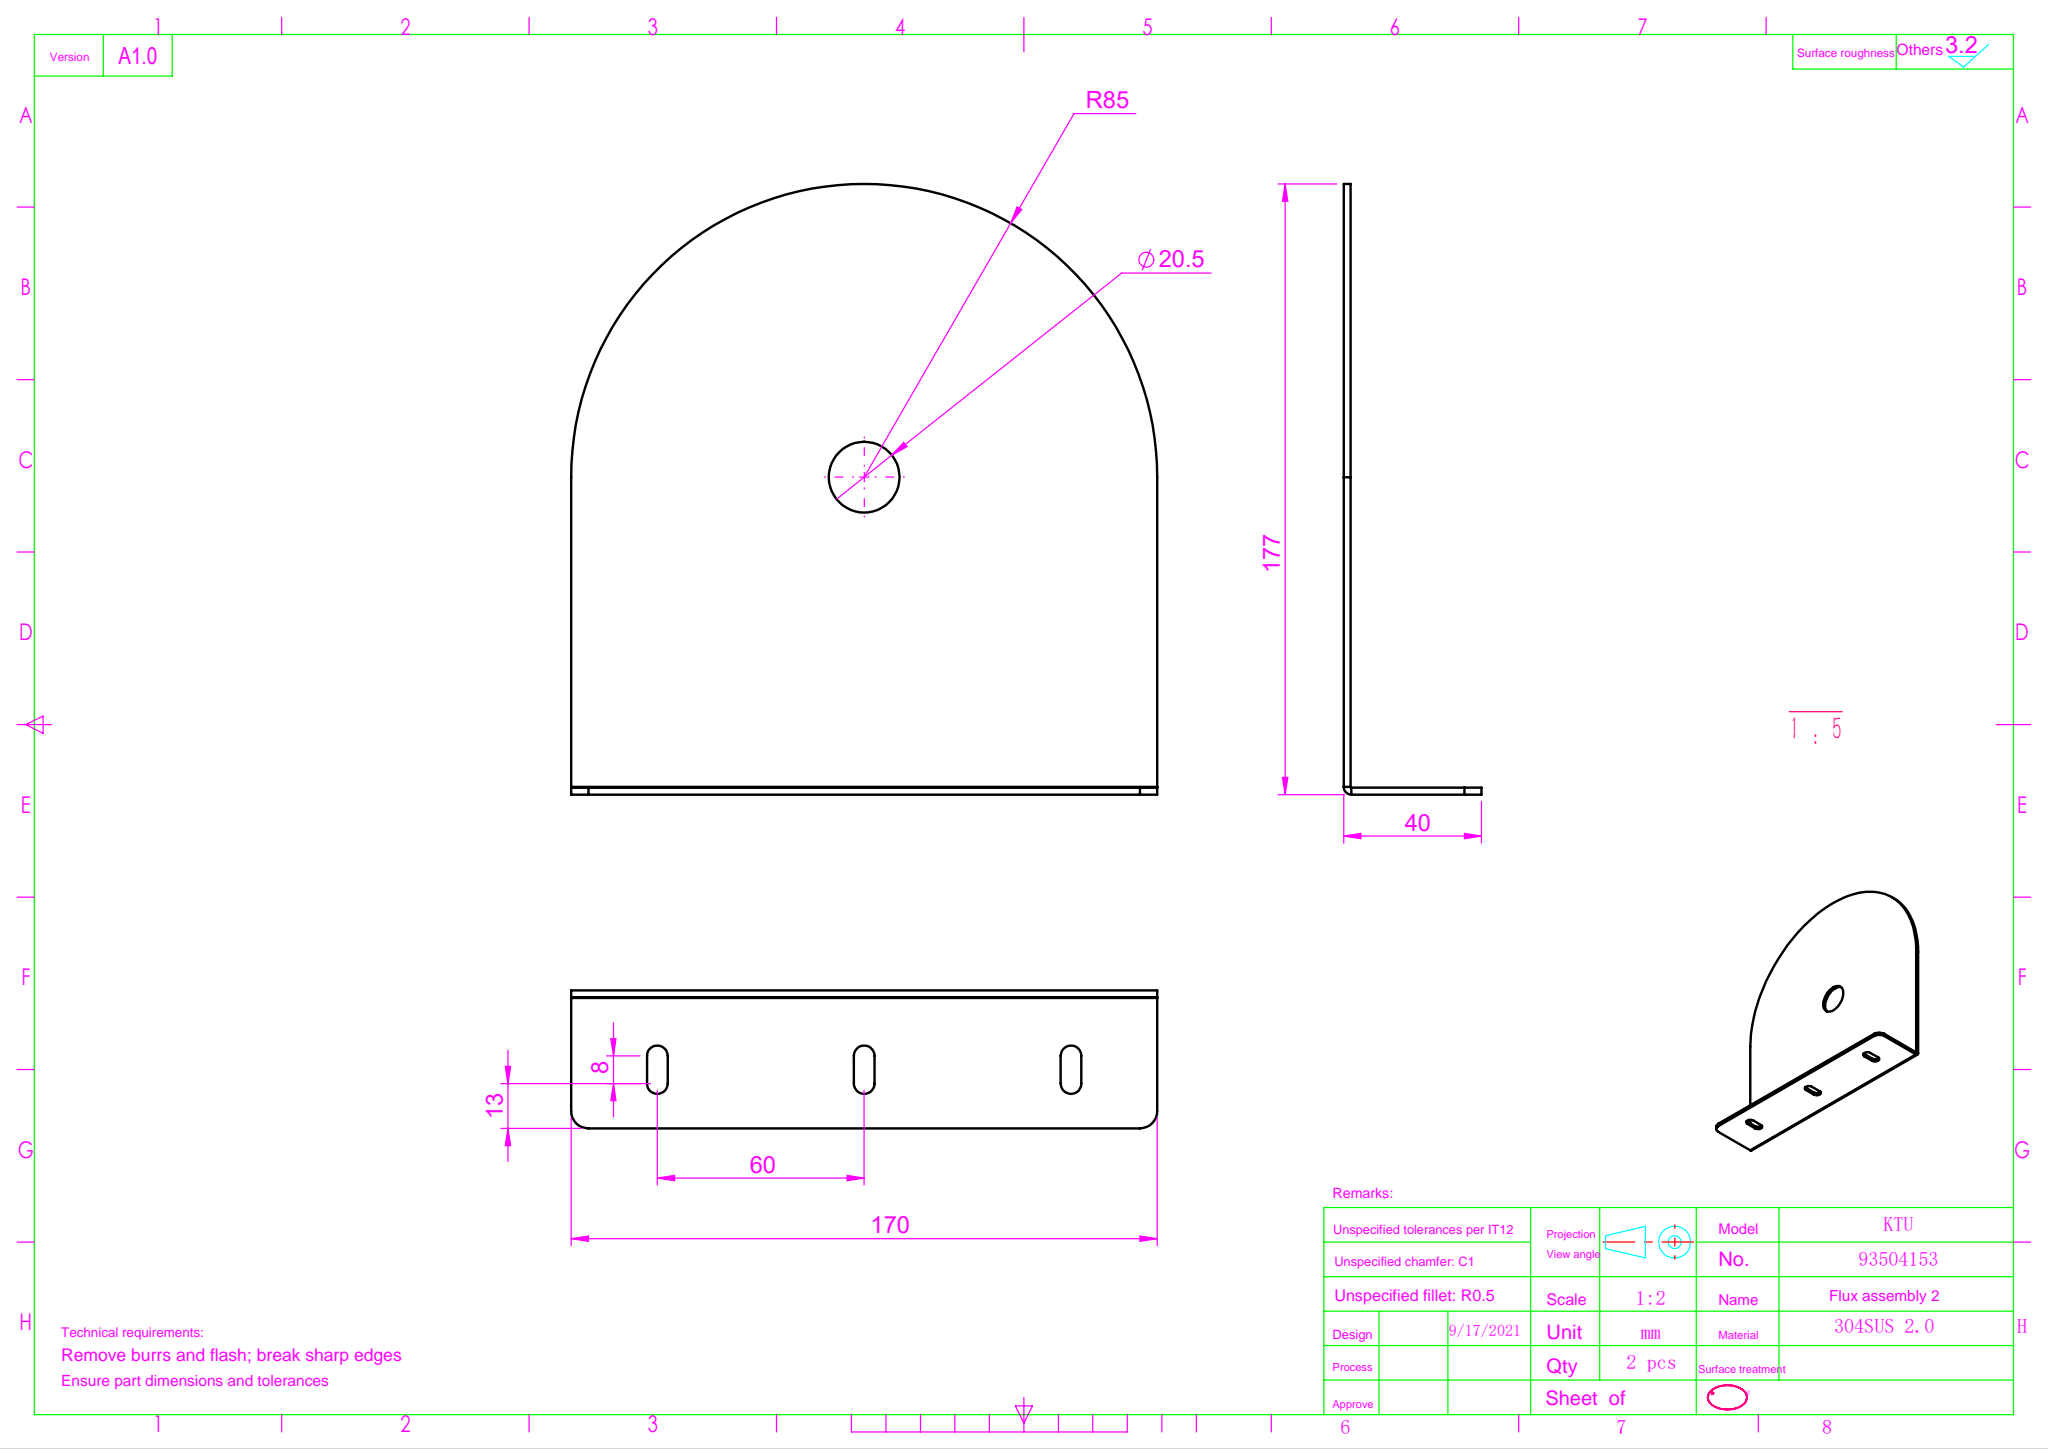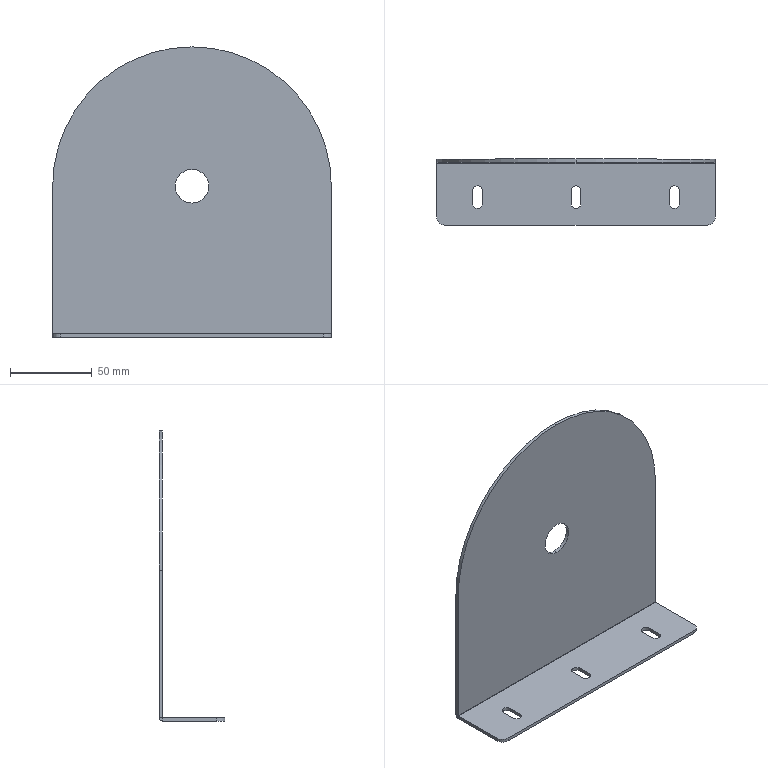Part | SolidWorks | features EdgeFlange 1, Fillet 1, FlatPattern 1, ICE 1, LPattern 1, SMBaseFlange 1, SheetMetal 1 | 1 solid | 31 faces | box 170 x 40 x 177 mm | volume 65584 mm3 | plane 17 | cylinder 14 | commonest cylinder face diameters 6 x6 10 x2 20.5 x2 170 x2 0.4 x1 4.4 x1
STEP:
#1=CARTESIAN_POINT('',(0.,-2.,-10.25));
#2=VERTEX_POINT('',#1);
#3=CARTESIAN_POINT('',(0.,-2.,10.25));
#4=VERTEX_POINT('',#3);
#5=CARTESIAN_POINT('',(0.,-2.,0.));
#6=DIRECTION('',(0.,1.,0.));
#7=DIRECTION('',(0.,0.,1.));
#8=AXIS2_PLACEMENT_3D('',#5,#6,#7);
#9=CIRCLE('',#8,10.25);
#10=EDGE_CURVE('',#2,#4,#9,.T.);
#11=ORIENTED_EDGE('',*,*,#10,.F.);
#12=CARTESIAN_POINT('',(0.,0.,-10.25));
#13=VERTEX_POINT('',#12);
#14=CARTESIAN_POINT('',(0.,-2.,-10.25));
#15=DIRECTION('',(0.,1.,0.));
#16=VECTOR('',#15,1000.);
#17=LINE('',#14,#16);
#18=EDGE_CURVE('',#2,#13,#17,.T.);
#19=ORIENTED_EDGE('',*,*,#18,.T.);
#20=CARTESIAN_POINT('',(0.,0.,10.25));
#21=VERTEX_POINT('',#20);
#22=CARTESIAN_POINT('',(0.,0.,0.));
#23=DIRECTION('',(0.,1.,0.));
#24=DIRECTION('',(0.,0.,1.));
#25=AXIS2_PLACEMENT_3D('',#22,#23,#24);
#26=CIRCLE('',#25,10.25);
#27=EDGE_CURVE('',#13,#21,#26,.T.);
#28=ORIENTED_EDGE('',*,*,#27,.T.);
#29=CARTESIAN_POINT('',(0.,-2.,10.25));
#30=DIRECTION('',(0.,1.,0.));
#31=VECTOR('',#30,1000.);
#32=LINE('',#29,#31);
#33=EDGE_CURVE('',#4,#21,#32,.T.);
#34=ORIENTED_EDGE('',*,*,#33,.F.);
#35=EDGE_LOOP('',(#11,#19,#28,#34));
#36=FACE_OUTER_BOUND('',#35,.T.);
#37=CARTESIAN_POINT('',(0.,-2.,0.));
#38=DIRECTION('',(0.,1.,0.));
#39=DIRECTION('',(0.,0.,1.));
#40=AXIS2_PLACEMENT_3D('',#37,#38,#39);
#41=CYLINDRICAL_SURFACE('',#40,10.25);
#42=ADVANCED_FACE('',(#36),#41,.F.);
#43=CARTESIAN_POINT('',(-85.,-2.,0.));
#44=VERTEX_POINT('',#43);
#45=CARTESIAN_POINT('',(0.,-2.,85.));
#46=VERTEX_POINT('',#45);
#47=CARTESIAN_POINT('',(0.,-2.,0.));
#48=DIRECTION('',(0.,1.,0.));
#49=DIRECTION('',(0.,0.,1.));
#50=AXIS2_PLACEMENT_3D('',#47,#48,#49);
#51=CIRCLE('',#50,85.);
#52=EDGE_CURVE('',#44,#46,#51,.T.);
#53=ORIENTED_EDGE('',*,*,#52,.T.);
#54=CARTESIAN_POINT('',(0.,0.,85.));
#55=VERTEX_POINT('',#54);
#56=CARTESIAN_POINT('',(0.,-2.,85.));
#57=DIRECTION('',(0.,1.,0.));
#58=VECTOR('',#57,1000.);
#59=LINE('',#56,#58);
#60=EDGE_CURVE('',#46,#55,#59,.T.);
#61=ORIENTED_EDGE('',*,*,#60,.T.);
#62=CARTESIAN_POINT('',(-85.,0.,0.));
#63=VERTEX_POINT('',#62);
#64=CARTESIAN_POINT('',(0.,0.,0.));
#65=DIRECTION('',(0.,1.,0.));
#66=DIRECTION('',(0.,0.,1.));
#67=AXIS2_PLACEMENT_3D('',#64,#65,#66);
#68=CIRCLE('',#67,85.);
#69=EDGE_CURVE('',#63,#55,#68,.T.);
#70=ORIENTED_EDGE('',*,*,#69,.F.);
#71=CARTESIAN_POINT('',(-85.,-2.,0.));
#72=DIRECTION('',(0.,1.,0.));
#73=VECTOR('',#72,1000.);
#74=LINE('',#71,#73);
#75=EDGE_CURVE('',#44,#63,#74,.T.);
#76=ORIENTED_EDGE('',*,*,#75,.F.);
#77=EDGE_LOOP('',(#53,#61,#70,#76));
#78=FACE_OUTER_BOUND('',#77,.T.);
#79=CARTESIAN_POINT('',(0.,-2.,0.));
#80=DIRECTION('',(0.,1.,0.));
#81=DIRECTION('',(0.,0.,1.));
#82=AXIS2_PLACEMENT_3D('',#79,#80,#81);
#83=CYLINDRICAL_SURFACE('',#82,85.);
#84=ADVANCED_FACE('',(#78),#83,.T.);
#85=CARTESIAN_POINT('',(85.,-2.,0.));
#86=VERTEX_POINT('',#85);
#87=CARTESIAN_POINT('',(85.,-2.,-89.8));
#88=VERTEX_POINT('',#87);
#89=CARTESIAN_POINT('',(85.,-2.,-92.));
#90=DIRECTION('',(0.,0.,-1.));
#91=VECTOR('',#90,1000.);
#92=LINE('',#89,#91);
#93=EDGE_CURVE('',#86,#88,#92,.T.);
#94=ORIENTED_EDGE('',*,*,#93,.T.);
#95=CARTESIAN_POINT('',(85.,0.,-89.8));
#96=VERTEX_POINT('',#95);
#97=CARTESIAN_POINT('',(85.,-2.,-89.8));
#98=DIRECTION('',(0.,1.,0.));
#99=VECTOR('',#98,1000.);
#100=LINE('',#97,#99);
#101=EDGE_CURVE('',#88,#96,#100,.T.);
#102=ORIENTED_EDGE('',*,*,#101,.T.);
#103=CARTESIAN_POINT('',(85.,0.,0.));
#104=VERTEX_POINT('',#103);
#105=CARTESIAN_POINT('',(85.,0.,-92.));
#106=DIRECTION('',(0.,0.,-1.));
#107=VECTOR('',#106,1000.);
#108=LINE('',#105,#107);
#109=EDGE_CURVE('',#104,#96,#108,.T.);
#110=ORIENTED_EDGE('',*,*,#109,.F.);
#111=CARTESIAN_POINT('',(85.,-2.,0.));
#112=DIRECTION('',(0.,1.,0.));
#113=VECTOR('',#112,1000.);
#114=LINE('',#111,#113);
#115=EDGE_CURVE('',#86,#104,#114,.T.);
#116=ORIENTED_EDGE('',*,*,#115,.F.);
#117=EDGE_LOOP('',(#94,#102,#110,#116));
#118=FACE_OUTER_BOUND('',#117,.T.);
#119=CARTESIAN_POINT('',(85.,-2.,-92.));
#120=DIRECTION('',(1.,0.,0.));
#121=DIRECTION('',(0.,0.,-1.));
#122=AXIS2_PLACEMENT_3D('',#119,#120,#121);
#123=PLANE('',#122);
#124=ADVANCED_FACE('',(#118),#123,.T.);
#125=CARTESIAN_POINT('',(0.,-2.,0.));
#126=DIRECTION('',(0.,1.,0.));
#127=DIRECTION('',(0.,0.,1.));
#128=AXIS2_PLACEMENT_3D('',#125,#126,#127);
#129=CIRCLE('',#128,10.25);
#130=EDGE_CURVE('',#4,#2,#129,.T.);
#131=ORIENTED_EDGE('',*,*,#130,.T.);
#132=ORIENTED_EDGE('',*,*,#10,.T.);
#133=EDGE_LOOP('',(#131,#132));
#134=FACE_BOUND('',#133,.T.);
#135=CARTESIAN_POINT('',(-85.,-2.,-89.8));
#136=VERTEX_POINT('',#135);
#137=CARTESIAN_POINT('',(85.,-2.,-89.8));
#138=DIRECTION('',(-1.,0.,0.));
#139=VECTOR('',#138,1000.);
#140=LINE('',#137,#139);
#141=EDGE_CURVE('',#88,#136,#140,.T.);
#142=ORIENTED_EDGE('',*,*,#141,.F.);
#143=ORIENTED_EDGE('',*,*,#93,.F.);
#144=CARTESIAN_POINT('',(0.,-2.,0.));
#145=DIRECTION('',(0.,1.,0.));
#146=DIRECTION('',(0.,0.,1.));
#147=AXIS2_PLACEMENT_3D('',#144,#145,#146);
#148=CIRCLE('',#147,85.);
#149=EDGE_CURVE('',#46,#86,#148,.T.);
#150=ORIENTED_EDGE('',*,*,#149,.F.);
#151=ORIENTED_EDGE('',*,*,#52,.F.);
#152=CARTESIAN_POINT('',(-85.,-2.,0.));
#153=DIRECTION('',(0.,0.,1.));
#154=VECTOR('',#153,1000.);
#155=LINE('',#152,#154);
#156=EDGE_CURVE('',#136,#44,#155,.T.);
#157=ORIENTED_EDGE('',*,*,#156,.F.);
#158=EDGE_LOOP('',(#142,#143,#150,#151,#157));
#159=FACE_OUTER_BOUND('',#158,.T.);
#160=CARTESIAN_POINT('',(0.,-2.,0.));
#161=DIRECTION('',(0.,1.,0.));
#162=DIRECTION('',(0.,0.,1.));
#163=AXIS2_PLACEMENT_3D('',#160,#161,#162);
#164=PLANE('',#163);
#165=ADVANCED_FACE('',(#134,#159),#164,.F.);
#166=CARTESIAN_POINT('',(0.,0.,0.));
#167=DIRECTION('',(0.,1.,0.));
#168=DIRECTION('',(0.,0.,1.));
#169=AXIS2_PLACEMENT_3D('',#166,#167,#168);
#170=CIRCLE('',#169,10.25);
#171=EDGE_CURVE('',#21,#13,#170,.T.);
#172=ORIENTED_EDGE('',*,*,#171,.F.);
#173=ORIENTED_EDGE('',*,*,#27,.F.);
#174=EDGE_LOOP('',(#172,#173));
#175=FACE_BOUND('',#174,.T.);
#176=ORIENTED_EDGE('',*,*,#109,.T.);
#177=CARTESIAN_POINT('',(-85.,0.,-89.8));
#178=VERTEX_POINT('',#177);
#179=CARTESIAN_POINT('',(85.,0.,-89.8));
#180=DIRECTION('',(-1.,0.,0.));
#181=VECTOR('',#180,1000.);
#182=LINE('',#179,#181);
#183=EDGE_CURVE('',#96,#178,#182,.T.);
#184=ORIENTED_EDGE('',*,*,#183,.T.);
#185=CARTESIAN_POINT('',(-85.,0.,0.));
#186=DIRECTION('',(0.,0.,1.));
#187=VECTOR('',#186,1000.);
#188=LINE('',#185,#187);
#189=EDGE_CURVE('',#178,#63,#188,.T.);
#190=ORIENTED_EDGE('',*,*,#189,.T.);
#191=ORIENTED_EDGE('',*,*,#69,.T.);
#192=CARTESIAN_POINT('',(0.,0.,0.));
#193=DIRECTION('',(0.,1.,0.));
#194=DIRECTION('',(0.,0.,1.));
#195=AXIS2_PLACEMENT_3D('',#192,#193,#194);
#196=CIRCLE('',#195,85.);
#197=EDGE_CURVE('',#55,#104,#196,.T.);
#198=ORIENTED_EDGE('',*,*,#197,.T.);
#199=EDGE_LOOP('',(#176,#184,#190,#191,#198));
#200=FACE_OUTER_BOUND('',#199,.T.);
#201=CARTESIAN_POINT('',(0.,0.,0.));
#202=DIRECTION('',(0.,1.,0.));
#203=DIRECTION('',(0.,0.,1.));
#204=AXIS2_PLACEMENT_3D('',#201,#202,#203);
#205=PLANE('',#204);
#206=ADVANCED_FACE('',(#175,#200),#205,.T.);
#207=ORIENTED_EDGE('',*,*,#60,.F.);
#208=ORIENTED_EDGE('',*,*,#149,.T.);
#209=ORIENTED_EDGE('',*,*,#115,.T.);
#210=ORIENTED_EDGE('',*,*,#197,.F.);
#211=EDGE_LOOP('',(#207,#208,#209,#210));
#212=FACE_OUTER_BOUND('',#211,.T.);
#213=CARTESIAN_POINT('',(0.,-2.,0.));
#214=DIRECTION('',(0.,1.,0.));
#215=DIRECTION('',(0.,0.,1.));
#216=AXIS2_PLACEMENT_3D('',#213,#214,#215);
#217=CYLINDRICAL_SURFACE('',#216,85.);
#218=ADVANCED_FACE('',(#212),#217,.T.);
#219=CARTESIAN_POINT('',(-85.,-2.,-89.8));
#220=DIRECTION('',(0.,1.,0.));
#221=VECTOR('',#220,1000.);
#222=LINE('',#219,#221);
#223=EDGE_CURVE('',#136,#178,#222,.T.);
#224=ORIENTED_EDGE('',*,*,#223,.F.);
#225=ORIENTED_EDGE('',*,*,#156,.T.);
#226=ORIENTED_EDGE('',*,*,#75,.T.);
#227=ORIENTED_EDGE('',*,*,#189,.F.);
#228=EDGE_LOOP('',(#224,#225,#226,#227));
#229=FACE_OUTER_BOUND('',#228,.T.);
#230=CARTESIAN_POINT('',(-85.,-2.,0.));
#231=DIRECTION('',(-1.,0.,0.));
#232=DIRECTION('',(0.,0.,1.));
#233=AXIS2_PLACEMENT_3D('',#230,#231,#232);
#234=PLANE('',#233);
#235=ADVANCED_FACE('',(#229),#234,.T.);
#236=ORIENTED_EDGE('',*,*,#18,.F.);
#237=ORIENTED_EDGE('',*,*,#130,.F.);
#238=ORIENTED_EDGE('',*,*,#33,.T.);
#239=ORIENTED_EDGE('',*,*,#171,.T.);
#240=EDGE_LOOP('',(#236,#237,#238,#239));
#241=FACE_OUTER_BOUND('',#240,.T.);
#242=CARTESIAN_POINT('',(0.,-2.,0.));
#243=DIRECTION('',(0.,1.,0.));
#244=DIRECTION('',(0.,0.,1.));
#245=AXIS2_PLACEMENT_3D('',#242,#243,#244);
#246=CYLINDRICAL_SURFACE('',#245,10.25);
#247=ADVANCED_FACE('',(#241),#246,.F.);
#248=CARTESIAN_POINT('',(-85.,-2.2,-90.));
#249=VERTEX_POINT('',#248);
#250=CARTESIAN_POINT('',(-85.,-2.2,-92.));
#251=VERTEX_POINT('',#250);
#252=CARTESIAN_POINT('',(-85.,-2.2,-92.));
#253=DIRECTION('',(0.,0.,-1.));
#254=VECTOR('',#253,1000.);
#255=LINE('',#252,#254);
#256=EDGE_CURVE('',#249,#251,#255,.T.);
#257=ORIENTED_EDGE('',*,*,#256,.F.);
#258=CARTESIAN_POINT('',(-85.,-2.2,-89.8));
#259=DIRECTION('',(-1.,0.,0.));
#260=DIRECTION('',(0.,0.,-1.));
#261=AXIS2_PLACEMENT_3D('',#258,#259,#260);
#262=CIRCLE('',#261,0.2);
#263=EDGE_CURVE('',#136,#249,#262,.T.);
#264=ORIENTED_EDGE('',*,*,#263,.F.);
#265=ORIENTED_EDGE('',*,*,#223,.T.);
#266=CARTESIAN_POINT('',(-85.,-2.2,-89.8));
#267=DIRECTION('',(-1.,0.,0.));
#268=DIRECTION('',(0.,0.,-1.));
#269=AXIS2_PLACEMENT_3D('',#266,#267,#268);
#270=CIRCLE('',#269,2.2);
#271=EDGE_CURVE('',#178,#251,#270,.T.);
#272=ORIENTED_EDGE('',*,*,#271,.T.);
#273=EDGE_LOOP('',(#257,#264,#265,#272));
#274=FACE_OUTER_BOUND('',#273,.T.);
#275=CARTESIAN_POINT('',(-85.,-2.2,-89.8));
#276=DIRECTION('',(-1.,0.,0.));
#277=DIRECTION('',(0.,0.,1.));
#278=AXIS2_PLACEMENT_3D('',#275,#276,#277);
#279=PLANE('',#278);
#280=ADVANCED_FACE('',(#274),#279,.T.);
#281=CARTESIAN_POINT('',(85.,-2.2,-90.));
#282=VERTEX_POINT('',#281);
#283=CARTESIAN_POINT('',(85.,-2.2,-89.8));
#284=DIRECTION('',(1.,0.,0.));
#285=DIRECTION('',(0.,0.,-1.));
#286=AXIS2_PLACEMENT_3D('',#283,#284,#285);
#287=CIRCLE('',#286,0.2);
#288=EDGE_CURVE('',#282,#88,#287,.T.);
#289=ORIENTED_EDGE('',*,*,#288,.F.);
#290=CARTESIAN_POINT('',(85.,-2.2,-92.));
#291=VERTEX_POINT('',#290);
#292=CARTESIAN_POINT('',(85.,-2.2,-90.));
#293=DIRECTION('',(0.,0.,-1.));
#294=VECTOR('',#293,1000.);
#295=LINE('',#292,#294);
#296=EDGE_CURVE('',#282,#291,#295,.T.);
#297=ORIENTED_EDGE('',*,*,#296,.T.);
#298=CARTESIAN_POINT('',(85.,-2.2,-89.8));
#299=DIRECTION('',(1.,0.,0.));
#300=DIRECTION('',(0.,0.,-1.));
#301=AXIS2_PLACEMENT_3D('',#298,#299,#300);
#302=CIRCLE('',#301,2.2);
#303=EDGE_CURVE('',#291,#96,#302,.T.);
#304=ORIENTED_EDGE('',*,*,#303,.T.);
#305=ORIENTED_EDGE('',*,*,#101,.F.);
#306=EDGE_LOOP('',(#289,#297,#304,#305));
#307=FACE_OUTER_BOUND('',#306,.T.);
#308=CARTESIAN_POINT('',(85.,-2.2,-89.8));
#309=DIRECTION('',(-1.,0.,0.));
#310=DIRECTION('',(0.,0.,1.));
#311=AXIS2_PLACEMENT_3D('',#308,#309,#310);
#312=PLANE('',#311);
#313=ADVANCED_FACE('',(#307),#312,.F.);
#314=ORIENTED_EDGE('',*,*,#183,.F.);
#315=ORIENTED_EDGE('',*,*,#303,.F.);
#316=CARTESIAN_POINT('',(0.,-2.2,-92.));
#317=DIRECTION('',(1.,0.,0.));
#318=VECTOR('',#317,1000.);
#319=LINE('',#316,#318);
#320=EDGE_CURVE('',#251,#291,#319,.T.);
#321=ORIENTED_EDGE('',*,*,#320,.F.);
#322=ORIENTED_EDGE('',*,*,#271,.F.);
#323=EDGE_LOOP('',(#314,#315,#321,#322));
#324=FACE_OUTER_BOUND('',#323,.T.);
#325=CARTESIAN_POINT('',(85.,-2.2,-89.8));
#326=DIRECTION('',(1.,0.,0.));
#327=DIRECTION('',(0.,0.,-1.));
#328=AXIS2_PLACEMENT_3D('',#325,#326,#327);
#329=CYLINDRICAL_SURFACE('',#328,2.2);
#330=ADVANCED_FACE('',(#324),#329,.T.);
#331=ORIENTED_EDGE('',*,*,#141,.T.);
#332=ORIENTED_EDGE('',*,*,#263,.T.);
#333=CARTESIAN_POINT('',(-85.,-2.2,-90.));
#334=DIRECTION('',(1.,0.,0.));
#335=VECTOR('',#334,1000.);
#336=LINE('',#333,#335);
#337=EDGE_CURVE('',#249,#282,#336,.T.);
#338=ORIENTED_EDGE('',*,*,#337,.T.);
#339=ORIENTED_EDGE('',*,*,#288,.T.);
#340=EDGE_LOOP('',(#331,#332,#338,#339));
#341=FACE_OUTER_BOUND('',#340,.T.);
#342=CARTESIAN_POINT('',(85.,-2.2,-89.8));
#343=DIRECTION('',(1.,0.,0.));
#344=DIRECTION('',(0.,0.,-1.));
#345=AXIS2_PLACEMENT_3D('',#342,#343,#344);
#346=CYLINDRICAL_SURFACE('',#345,0.2);
#347=ADVANCED_FACE('',(#341),#346,.F.);
#348=CARTESIAN_POINT('',(85.,-35.,-90.));
#349=VERTEX_POINT('',#348);
#350=CARTESIAN_POINT('',(85.,0.,-90.));
#351=DIRECTION('',(0.,1.,0.));
#352=VECTOR('',#351,1000.);
#353=LINE('',#350,#352);
#354=EDGE_CURVE('',#349,#282,#353,.T.);
#355=ORIENTED_EDGE('',*,*,#354,.F.);
#356=CARTESIAN_POINT('',(85.,-35.,-92.));
#357=VERTEX_POINT('',#356);
#358=CARTESIAN_POINT('',(85.,-35.,-92.));
#359=DIRECTION('',(0.,0.,-1.));
#360=VECTOR('',#359,1000.);
#361=LINE('',#358,#360);
#362=EDGE_CURVE('',#349,#357,#361,.T.);
#363=ORIENTED_EDGE('',*,*,#362,.T.);
#364=CARTESIAN_POINT('',(85.,-2.,-92.));
#365=DIRECTION('',(0.,1.,0.));
#366=VECTOR('',#365,1000.);
#367=LINE('',#364,#366);
#368=EDGE_CURVE('',#357,#291,#367,.T.);
#369=ORIENTED_EDGE('',*,*,#368,.T.);
#370=ORIENTED_EDGE('',*,*,#296,.F.);
#371=EDGE_LOOP('',(#355,#363,#369,#370));
#372=FACE_OUTER_BOUND('',#371,.T.);
#373=CARTESIAN_POINT('',(85.,-2.,-92.));
#374=DIRECTION('',(1.,0.,0.));
#375=DIRECTION('',(0.,0.,-1.));
#376=AXIS2_PLACEMENT_3D('',#373,#374,#375);
#377=PLANE('',#376);
#378=ADVANCED_FACE('',(#372),#377,.T.);
#379=CARTESIAN_POINT('',(-85.,-35.,-92.));
#380=VERTEX_POINT('',#379);
#381=CARTESIAN_POINT('',(-85.,-40.,-92.));
#382=DIRECTION('',(0.,-1.,0.));
#383=VECTOR('',#382,1000.);
#384=LINE('',#381,#383);
#385=EDGE_CURVE('',#251,#380,#384,.T.);
#386=ORIENTED_EDGE('',*,*,#385,.T.);
#387=CARTESIAN_POINT('',(-85.,-35.,-90.));
#388=VERTEX_POINT('',#387);
#389=CARTESIAN_POINT('',(-85.,-35.,-92.));
#390=DIRECTION('',(0.,0.,1.));
#391=VECTOR('',#390,1000.);
#392=LINE('',#389,#391);
#393=EDGE_CURVE('',#380,#388,#392,.T.);
#394=ORIENTED_EDGE('',*,*,#393,.T.);
#395=CARTESIAN_POINT('',(-85.,0.,-90.));
#396=DIRECTION('',(0.,-1.,0.));
#397=VECTOR('',#396,1000.);
#398=LINE('',#395,#397);
#399=EDGE_CURVE('',#249,#388,#398,.T.);
#400=ORIENTED_EDGE('',*,*,#399,.F.);
#401=ORIENTED_EDGE('',*,*,#256,.T.);
#402=EDGE_LOOP('',(#386,#394,#400,#401));
#403=FACE_OUTER_BOUND('',#402,.T.);
#404=CARTESIAN_POINT('',(-85.,-40.,-92.));
#405=DIRECTION('',(-1.,0.,0.));
#406=DIRECTION('',(0.,0.,1.));
#407=AXIS2_PLACEMENT_3D('',#404,#405,#406);
#408=PLANE('',#407);
#409=ADVANCED_FACE('',(#403),#408,.T.);
#410=CARTESIAN_POINT('',(-57.,-19.,-92.));
#411=VERTEX_POINT('',#410);
#412=CARTESIAN_POINT('',(-63.,-19.,-92.));
#413=VERTEX_POINT('',#412);
#414=CARTESIAN_POINT('',(-60.,-19.,-92.));
#415=DIRECTION('',(0.,0.,1.));
#416=DIRECTION('',(1.,0.,0.));
#417=AXIS2_PLACEMENT_3D('',#414,#415,#416);
#418=CIRCLE('',#417,3.);
#419=EDGE_CURVE('',#411,#413,#418,.T.);
#420=ORIENTED_EDGE('',*,*,#419,.T.);
#421=CARTESIAN_POINT('',(-63.,-27.,-92.));
#422=VERTEX_POINT('',#421);
#423=CARTESIAN_POINT('',(-63.,-19.,-92.));
#424=DIRECTION('',(0.,-1.,0.));
#425=VECTOR('',#424,1000.);
#426=LINE('',#423,#425);
#427=EDGE_CURVE('',#413,#422,#426,.T.);
#428=ORIENTED_EDGE('',*,*,#427,.T.);
#429=CARTESIAN_POINT('',(-57.,-27.,-92.));
#430=VERTEX_POINT('',#429);
#431=CARTESIAN_POINT('',(-60.,-27.,-92.));
#432=DIRECTION('',(0.,0.,1.));
#433=DIRECTION('',(1.,0.,0.));
#434=AXIS2_PLACEMENT_3D('',#431,#432,#433);
#435=CIRCLE('',#434,3.);
#436=EDGE_CURVE('',#422,#430,#435,.T.);
#437=ORIENTED_EDGE('',*,*,#436,.T.);
#438=CARTESIAN_POINT('',(-57.,-19.,-92.));
#439=DIRECTION('',(0.,1.,0.));
#440=VECTOR('',#439,1000.);
#441=LINE('',#438,#440);
#442=EDGE_CURVE('',#430,#411,#441,.T.);
#443=ORIENTED_EDGE('',*,*,#442,.T.);
#444=EDGE_LOOP('',(#420,#428,#437,#443));
#445=FACE_BOUND('',#444,.T.);
#446=CARTESIAN_POINT('',(63.,-19.,-92.));
#447=VERTEX_POINT('',#446);
#448=CARTESIAN_POINT('',(57.,-19.,-92.));
#449=VERTEX_POINT('',#448);
#450=CARTESIAN_POINT('',(60.,-19.,-92.));
#451=DIRECTION('',(0.,0.,1.));
#452=DIRECTION('',(1.,0.,0.));
#453=AXIS2_PLACEMENT_3D('',#450,#451,#452);
#454=CIRCLE('',#453,3.);
#455=EDGE_CURVE('',#447,#449,#454,.T.);
#456=ORIENTED_EDGE('',*,*,#455,.T.);
#457=CARTESIAN_POINT('',(57.,-27.,-92.));
#458=VERTEX_POINT('',#457);
#459=CARTESIAN_POINT('',(57.,-19.,-92.));
#460=DIRECTION('',(0.,-1.,0.));
#461=VECTOR('',#460,1000.);
#462=LINE('',#459,#461);
#463=EDGE_CURVE('',#449,#458,#462,.T.);
#464=ORIENTED_EDGE('',*,*,#463,.T.);
#465=CARTESIAN_POINT('',(63.,-27.,-92.));
#466=VERTEX_POINT('',#465);
#467=CARTESIAN_POINT('',(60.,-27.,-92.));
#468=DIRECTION('',(0.,0.,1.));
#469=DIRECTION('',(1.,0.,0.));
#470=AXIS2_PLACEMENT_3D('',#467,#468,#469);
#471=CIRCLE('',#470,3.);
#472=EDGE_CURVE('',#458,#466,#471,.T.);
#473=ORIENTED_EDGE('',*,*,#472,.T.);
#474=CARTESIAN_POINT('',(63.,-19.,-92.));
#475=DIRECTION('',(0.,1.,0.));
#476=VECTOR('',#475,1000.);
#477=LINE('',#474,#476);
#478=EDGE_CURVE('',#466,#447,#477,.T.);
#479=ORIENTED_EDGE('',*,*,#478,.T.);
#480=EDGE_LOOP('',(#456,#464,#473,#479));
#481=FACE_BOUND('',#480,.T.);
#482=CARTESIAN_POINT('',(3.,-19.,-92.));
#483=VERTEX_POINT('',#482);
#484=CARTESIAN_POINT('',(-3.,-19.,-92.));
#485=VERTEX_POINT('',#484);
#486=CARTESIAN_POINT('',(0.,-19.,-92.));
#487=DIRECTION('',(0.,0.,1.));
#488=DIRECTION('',(1.,0.,0.));
#489=AXIS2_PLACEMENT_3D('',#486,#487,#488);
#490=CIRCLE('',#489,3.);
#491=EDGE_CURVE('',#483,#485,#490,.T.);
#492=ORIENTED_EDGE('',*,*,#491,.T.);
#493=CARTESIAN_POINT('',(-3.,-27.,-92.));
#494=VERTEX_POINT('',#493);
#495=CARTESIAN_POINT('',(-3.,-19.,-92.));
#496=DIRECTION('',(0.,-1.,0.));
#497=VECTOR('',#496,1000.);
#498=LINE('',#495,#497);
#499=EDGE_CURVE('',#485,#494,#498,.T.);
#500=ORIENTED_EDGE('',*,*,#499,.T.);
#501=CARTESIAN_POINT('',(3.,-27.,-92.));
#502=VERTEX_POINT('',#501);
#503=CARTESIAN_POINT('',(0.,-27.,-92.));
#504=DIRECTION('',(0.,0.,1.));
#505=DIRECTION('',(1.,0.,0.));
#506=AXIS2_PLACEMENT_3D('',#503,#504,#505);
#507=CIRCLE('',#506,3.);
#508=EDGE_CURVE('',#494,#502,#507,.T.);
#509=ORIENTED_EDGE('',*,*,#508,.T.);
#510=CARTESIAN_POINT('',(3.,-19.,-92.));
#511=DIRECTION('',(0.,1.,0.));
#512=VECTOR('',#511,1000.);
#513=LINE('',#510,#512);
#514=EDGE_CURVE('',#502,#483,#513,.T.);
#515=ORIENTED_EDGE('',*,*,#514,.T.);
#516=EDGE_LOOP('',(#492,#500,#509,#515));
#517=FACE_BOUND('',#516,.T.);
#518=CARTESIAN_POINT('',(-80.,-40.,-92.));
#519=VERTEX_POINT('',#518);
#520=CARTESIAN_POINT('',(80.,-40.,-92.));
#521=VERTEX_POINT('',#520);
#522=CARTESIAN_POINT('',(85.,-40.,-92.));
#523=DIRECTION('',(1.,0.,0.));
#524=VECTOR('',#523,1000.);
#525=LINE('',#522,#524);
#526=EDGE_CURVE('',#519,#521,#525,.T.);
#527=ORIENTED_EDGE('',*,*,#526,.F.);
#528=CARTESIAN_POINT('',(-80.,-35.,-92.));
#529=DIRECTION('',(0.,0.,-1.));
#530=DIRECTION('',(0.,1.,0.));
#531=AXIS2_PLACEMENT_3D('',#528,#529,#530);
#532=CIRCLE('',#531,5.);
#533=EDGE_CURVE('',#519,#380,#532,.T.);
#534=ORIENTED_EDGE('',*,*,#533,.T.);
#535=ORIENTED_EDGE('',*,*,#385,.F.);
#536=ORIENTED_EDGE('',*,*,#320,.T.);
#537=ORIENTED_EDGE('',*,*,#368,.F.);
#538=CARTESIAN_POINT('',(80.,-35.,-92.));
#539=DIRECTION('',(0.,0.,-1.));
#540=DIRECTION('',(0.,1.,0.));
#541=AXIS2_PLACEMENT_3D('',#538,#539,#540);
#542=CIRCLE('',#541,5.);
#543=EDGE_CURVE('',#357,#521,#542,.T.);
#544=ORIENTED_EDGE('',*,*,#543,.T.);
#545=EDGE_LOOP('',(#527,#534,#535,#536,#537,#544));
#546=FACE_OUTER_BOUND('',#545,.T.);
#547=CARTESIAN_POINT('',(0.,0.,-92.));
#548=DIRECTION('',(0.,0.,-1.));
#549=DIRECTION('',(0.,1.,0.));
#550=AXIS2_PLACEMENT_3D('',#547,#548,#549);
#551=PLANE('',#550);
#552=ADVANCED_FACE('',(#445,#481,#517,#546),#551,.T.);
#553=CARTESIAN_POINT('',(-63.,-19.,-90.));
#554=VERTEX_POINT('',#553);
#555=CARTESIAN_POINT('',(-63.,-27.,-90.));
#556=VERTEX_POINT('',#555);
#557=CARTESIAN_POINT('',(-63.,-19.,-90.));
#558=DIRECTION('',(0.,-1.,0.));
#559=VECTOR('',#558,1000.);
#560=LINE('',#557,#559);
#561=EDGE_CURVE('',#554,#556,#560,.T.);
#562=ORIENTED_EDGE('',*,*,#561,.F.);
#563=CARTESIAN_POINT('',(-57.,-19.,-90.));
#564=VERTEX_POINT('',#563);
#565=CARTESIAN_POINT('',(-60.,-19.,-90.));
#566=DIRECTION('',(0.,0.,1.));
#567=DIRECTION('',(1.,0.,0.));
#568=AXIS2_PLACEMENT_3D('',#565,#566,#567);
#569=CIRCLE('',#568,3.);
#570=EDGE_CURVE('',#564,#554,#569,.T.);
#571=ORIENTED_EDGE('',*,*,#570,.F.);
#572=CARTESIAN_POINT('',(-57.,-27.,-90.));
#573=VERTEX_POINT('',#572);
#574=CARTESIAN_POINT('',(-57.,-19.,-90.));
#575=DIRECTION('',(0.,1.,0.));
#576=VECTOR('',#575,1000.);
#577=LINE('',#574,#576);
#578=EDGE_CURVE('',#573,#564,#577,.T.);
#579=ORIENTED_EDGE('',*,*,#578,.F.);
#580=CARTESIAN_POINT('',(-60.,-27.,-90.));
#581=DIRECTION('',(0.,0.,1.));
#582=DIRECTION('',(1.,0.,0.));
#583=AXIS2_PLACEMENT_3D('',#580,#581,#582);
#584=CIRCLE('',#583,3.);
#585=EDGE_CURVE('',#556,#573,#584,.T.);
#586=ORIENTED_EDGE('',*,*,#585,.F.);
#587=EDGE_LOOP('',(#562,#571,#579,#586));
#588=FACE_BOUND('',#587,.T.);
#589=CARTESIAN_POINT('',(57.,-19.,-90.));
#590=VERTEX_POINT('',#589);
#591=CARTESIAN_POINT('',(57.,-27.,-90.));
#592=VERTEX_POINT('',#591);
#593=CARTESIAN_POINT('',(57.,-19.,-90.));
#594=DIRECTION('',(0.,-1.,0.));
#595=VECTOR('',#594,1000.);
#596=LINE('',#593,#595);
#597=EDGE_CURVE('',#590,#592,#596,.T.);
#598=ORIENTED_EDGE('',*,*,#597,.F.);
#599=CARTESIAN_POINT('',(63.,-19.,-90.));
#600=VERTEX_POINT('',#599);
#601=CARTESIAN_POINT('',(60.,-19.,-90.));
#602=DIRECTION('',(0.,0.,1.));
#603=DIRECTION('',(1.,0.,0.));
#604=AXIS2_PLACEMENT_3D('',#601,#602,#603);
#605=CIRCLE('',#604,3.);
#606=EDGE_CURVE('',#600,#590,#605,.T.);
#607=ORIENTED_EDGE('',*,*,#606,.F.);
#608=CARTESIAN_POINT('',(63.,-27.,-90.));
#609=VERTEX_POINT('',#608);
#610=CARTESIAN_POINT('',(63.,-19.,-90.));
#611=DIRECTION('',(0.,1.,0.));
#612=VECTOR('',#611,1000.);
#613=LINE('',#610,#612);
#614=EDGE_CURVE('',#609,#600,#613,.T.);
#615=ORIENTED_EDGE('',*,*,#614,.F.);
#616=CARTESIAN_POINT('',(60.,-27.,-90.));
#617=DIRECTION('',(0.,0.,1.));
#618=DIRECTION('',(1.,0.,0.));
#619=AXIS2_PLACEMENT_3D('',#616,#617,#618);
#620=CIRCLE('',#619,3.);
#621=EDGE_CURVE('',#592,#609,#620,.T.);
#622=ORIENTED_EDGE('',*,*,#621,.F.);
#623=EDGE_LOOP('',(#598,#607,#615,#622));
#624=FACE_BOUND('',#623,.T.);
#625=CARTESIAN_POINT('',(-3.,-19.,-90.));
#626=VERTEX_POINT('',#625);
#627=CARTESIAN_POINT('',(-3.,-27.,-90.));
#628=VERTEX_POINT('',#627);
#629=CARTESIAN_POINT('',(-3.,-19.,-90.));
#630=DIRECTION('',(0.,-1.,0.));
#631=VECTOR('',#630,1000.);
#632=LINE('',#629,#631);
#633=EDGE_CURVE('',#626,#628,#632,.T.);
#634=ORIENTED_EDGE('',*,*,#633,.F.);
#635=CARTESIAN_POINT('',(3.,-19.,-90.));
#636=VERTEX_POINT('',#635);
#637=CARTESIAN_POINT('',(0.,-19.,-90.));
#638=DIRECTION('',(0.,0.,1.));
#639=DIRECTION('',(1.,0.,0.));
#640=AXIS2_PLACEMENT_3D('',#637,#638,#639);
#641=CIRCLE('',#640,3.);
#642=EDGE_CURVE('',#636,#626,#641,.T.);
#643=ORIENTED_EDGE('',*,*,#642,.F.);
#644=CARTESIAN_POINT('',(3.,-27.,-90.));
#645=VERTEX_POINT('',#644);
#646=CARTESIAN_POINT('',(3.,-19.,-90.));
#647=DIRECTION('',(0.,1.,0.));
#648=VECTOR('',#647,1000.);
#649=LINE('',#646,#648);
#650=EDGE_CURVE('',#645,#636,#649,.T.);
#651=ORIENTED_EDGE('',*,*,#650,.F.);
#652=CARTESIAN_POINT('',(0.,-27.,-90.));
#653=DIRECTION('',(0.,0.,1.));
#654=DIRECTION('',(1.,0.,0.));
#655=AXIS2_PLACEMENT_3D('',#652,#653,#654);
#656=CIRCLE('',#655,3.);
#657=EDGE_CURVE('',#628,#645,#656,.T.);
#658=ORIENTED_EDGE('',*,*,#657,.F.);
#659=EDGE_LOOP('',(#634,#643,#651,#658));
#660=FACE_BOUND('',#659,.T.);
#661=ORIENTED_EDGE('',*,*,#399,.T.);
#662=CARTESIAN_POINT('',(-80.,-40.,-90.));
#663=VERTEX_POINT('',#662);
#664=CARTESIAN_POINT('',(-80.,-35.,-90.));
#665=DIRECTION('',(0.,0.,1.));
#666=DIRECTION('',(0.,1.,0.));
#667=AXIS2_PLACEMENT_3D('',#664,#665,#666);
#668=CIRCLE('',#667,5.);
#669=EDGE_CURVE('',#388,#663,#668,.T.);
#670=ORIENTED_EDGE('',*,*,#669,.T.);
#671=CARTESIAN_POINT('',(80.,-40.,-90.));
#672=VERTEX_POINT('',#671);
#673=CARTESIAN_POINT('',(0.,-40.,-90.));
#674=DIRECTION('',(1.,0.,0.));
#675=VECTOR('',#674,1000.);
#676=LINE('',#673,#675);
#677=EDGE_CURVE('',#663,#672,#676,.T.);
#678=ORIENTED_EDGE('',*,*,#677,.T.);
#679=CARTESIAN_POINT('',(80.,-35.,-90.));
#680=DIRECTION('',(0.,0.,1.));
#681=DIRECTION('',(0.,1.,0.));
#682=AXIS2_PLACEMENT_3D('',#679,#680,#681);
#683=CIRCLE('',#682,5.);
#684=EDGE_CURVE('',#672,#349,#683,.T.);
#685=ORIENTED_EDGE('',*,*,#684,.T.);
#686=ORIENTED_EDGE('',*,*,#354,.T.);
#687=ORIENTED_EDGE('',*,*,#337,.F.);
#688=EDGE_LOOP('',(#661,#670,#678,#685,#686,#687));
#689=FACE_OUTER_BOUND('',#688,.T.);
#690=CARTESIAN_POINT('',(0.,0.,-90.));
#691=DIRECTION('',(0.,0.,-1.));
#692=DIRECTION('',(0.,1.,0.));
#693=AXIS2_PLACEMENT_3D('',#690,#691,#692);
#694=PLANE('',#693);
#695=ADVANCED_FACE('',(#588,#624,#660,#689),#694,.F.);
#696=ORIENTED_EDGE('',*,*,#677,.F.);
#697=CARTESIAN_POINT('',(-80.,-40.,-92.));
#698=DIRECTION('',(0.,0.,-1.));
#699=VECTOR('',#698,1000.);
#700=LINE('',#697,#699);
#701=EDGE_CURVE('',#663,#519,#700,.T.);
#702=ORIENTED_EDGE('',*,*,#701,.T.);
#703=ORIENTED_EDGE('',*,*,#526,.T.);
#704=CARTESIAN_POINT('',(80.,-40.,-92.));
#705=DIRECTION('',(0.,0.,1.));
#706=VECTOR('',#705,1000.);
#707=LINE('',#704,#706);
#708=EDGE_CURVE('',#521,#672,#707,.T.);
#709=ORIENTED_EDGE('',*,*,#708,.T.);
#710=EDGE_LOOP('',(#696,#702,#703,#709));
#711=FACE_OUTER_BOUND('',#710,.T.);
#712=CARTESIAN_POINT('',(85.,-40.,-92.));
#713=DIRECTION('',(0.,-1.,0.));
#714=DIRECTION('',(0.,0.,-1.));
#715=AXIS2_PLACEMENT_3D('',#712,#713,#714);
#716=PLANE('',#715);
#717=ADVANCED_FACE('',(#711),#716,.T.);
#718=ORIENTED_EDGE('',*,*,#642,.T.);
#719=CARTESIAN_POINT('',(-3.,-19.,-92.));
#720=DIRECTION('',(0.,0.,1.));
#721=VECTOR('',#720,1000.);
#722=LINE('',#719,#721);
#723=EDGE_CURVE('',#485,#626,#722,.T.);
#724=ORIENTED_EDGE('',*,*,#723,.F.);
#725=ORIENTED_EDGE('',*,*,#491,.F.);
#726=CARTESIAN_POINT('',(3.,-19.,-92.));
#727=DIRECTION('',(0.,0.,1.));
#728=VECTOR('',#727,1000.);
#729=LINE('',#726,#728);
#730=EDGE_CURVE('',#483,#636,#729,.T.);
#731=ORIENTED_EDGE('',*,*,#730,.T.);
#732=EDGE_LOOP('',(#718,#724,#725,#731));
#733=FACE_OUTER_BOUND('',#732,.T.);
#734=CARTESIAN_POINT('',(0.,-19.,-92.));
#735=DIRECTION('',(0.,0.,1.));
#736=DIRECTION('',(1.,0.,0.));
#737=AXIS2_PLACEMENT_3D('',#734,#735,#736);
#738=CYLINDRICAL_SURFACE('',#737,3.);
#739=ADVANCED_FACE('',(#733),#738,.F.);
#740=ORIENTED_EDGE('',*,*,#650,.T.);
#741=ORIENTED_EDGE('',*,*,#730,.F.);
#742=ORIENTED_EDGE('',*,*,#514,.F.);
#743=CARTESIAN_POINT('',(3.,-27.,-92.));
#744=DIRECTION('',(0.,0.,1.));
#745=VECTOR('',#744,1000.);
#746=LINE('',#743,#745);
#747=EDGE_CURVE('',#502,#645,#746,.T.);
#748=ORIENTED_EDGE('',*,*,#747,.T.);
#749=EDGE_LOOP('',(#740,#741,#742,#748));
#750=FACE_OUTER_BOUND('',#749,.T.);
#751=CARTESIAN_POINT('',(3.,-19.,-92.));
#752=DIRECTION('',(1.,0.,0.));
#753=DIRECTION('',(0.,1.,0.));
#754=AXIS2_PLACEMENT_3D('',#751,#752,#753);
#755=PLANE('',#754);
#756=ADVANCED_FACE('',(#750),#755,.F.);
#757=ORIENTED_EDGE('',*,*,#657,.T.);
#758=ORIENTED_EDGE('',*,*,#747,.F.);
#759=ORIENTED_EDGE('',*,*,#508,.F.);
#760=CARTESIAN_POINT('',(-3.,-27.,-92.));
#761=DIRECTION('',(0.,0.,1.));
#762=VECTOR('',#761,1000.);
#763=LINE('',#760,#762);
#764=EDGE_CURVE('',#494,#628,#763,.T.);
#765=ORIENTED_EDGE('',*,*,#764,.T.);
#766=EDGE_LOOP('',(#757,#758,#759,#765));
#767=FACE_OUTER_BOUND('',#766,.T.);
#768=CARTESIAN_POINT('',(0.,-27.,-92.));
#769=DIRECTION('',(0.,0.,1.));
#770=DIRECTION('',(1.,0.,0.));
#771=AXIS2_PLACEMENT_3D('',#768,#769,#770);
#772=CYLINDRICAL_SURFACE('',#771,3.);
#773=ADVANCED_FACE('',(#767),#772,.F.);
#774=ORIENTED_EDGE('',*,*,#633,.T.);
#775=ORIENTED_EDGE('',*,*,#764,.F.);
#776=ORIENTED_EDGE('',*,*,#499,.F.);
#777=ORIENTED_EDGE('',*,*,#723,.T.);
#778=EDGE_LOOP('',(#774,#775,#776,#777));
#779=FACE_OUTER_BOUND('',#778,.T.);
#780=CARTESIAN_POINT('',(-3.,-19.,-92.));
#781=DIRECTION('',(-1.,0.,0.));
#782=DIRECTION('',(0.,-1.,0.));
#783=AXIS2_PLACEMENT_3D('',#780,#781,#782);
#784=PLANE('',#783);
#785=ADVANCED_FACE('',(#779),#784,.F.);
#786=ORIENTED_EDGE('',*,*,#606,.T.);
#787=CARTESIAN_POINT('',(57.,-19.,-92.));
#788=DIRECTION('',(0.,0.,1.));
#789=VECTOR('',#788,1000.);
#790=LINE('',#787,#789);
#791=EDGE_CURVE('',#449,#590,#790,.T.);
#792=ORIENTED_EDGE('',*,*,#791,.F.);
#793=ORIENTED_EDGE('',*,*,#455,.F.);
#794=CARTESIAN_POINT('',(63.,-19.,-92.));
#795=DIRECTION('',(0.,0.,1.));
#796=VECTOR('',#795,1000.);
#797=LINE('',#794,#796);
#798=EDGE_CURVE('',#447,#600,#797,.T.);
#799=ORIENTED_EDGE('',*,*,#798,.T.);
#800=EDGE_LOOP('',(#786,#792,#793,#799));
#801=FACE_OUTER_BOUND('',#800,.T.);
#802=CARTESIAN_POINT('',(60.,-19.,-92.));
#803=DIRECTION('',(0.,0.,1.));
#804=DIRECTION('',(1.,0.,0.));
#805=AXIS2_PLACEMENT_3D('',#802,#803,#804);
#806=CYLINDRICAL_SURFACE('',#805,3.);
#807=ADVANCED_FACE('',(#801),#806,.F.);
#808=ORIENTED_EDGE('',*,*,#614,.T.);
#809=ORIENTED_EDGE('',*,*,#798,.F.);
#810=ORIENTED_EDGE('',*,*,#478,.F.);
#811=CARTESIAN_POINT('',(63.,-27.,-92.));
#812=DIRECTION('',(0.,0.,1.));
#813=VECTOR('',#812,1000.);
#814=LINE('',#811,#813);
#815=EDGE_CURVE('',#466,#609,#814,.T.);
#816=ORIENTED_EDGE('',*,*,#815,.T.);
#817=EDGE_LOOP('',(#808,#809,#810,#816));
#818=FACE_OUTER_BOUND('',#817,.T.);
#819=CARTESIAN_POINT('',(63.,-19.,-92.));
#820=DIRECTION('',(1.,0.,0.));
#821=DIRECTION('',(0.,1.,0.));
#822=AXIS2_PLACEMENT_3D('',#819,#820,#821);
#823=PLANE('',#822);
#824=ADVANCED_FACE('',(#818),#823,.F.);
#825=ORIENTED_EDGE('',*,*,#621,.T.);
#826=ORIENTED_EDGE('',*,*,#815,.F.);
#827=ORIENTED_EDGE('',*,*,#472,.F.);
#828=CARTESIAN_POINT('',(57.,-27.,-92.));
#829=DIRECTION('',(0.,0.,1.));
#830=VECTOR('',#829,1000.);
#831=LINE('',#828,#830);
#832=EDGE_CURVE('',#458,#592,#831,.T.);
#833=ORIENTED_EDGE('',*,*,#832,.T.);
#834=EDGE_LOOP('',(#825,#826,#827,#833));
#835=FACE_OUTER_BOUND('',#834,.T.);
#836=CARTESIAN_POINT('',(60.,-27.,-92.));
#837=DIRECTION('',(0.,0.,1.));
#838=DIRECTION('',(1.,0.,0.));
#839=AXIS2_PLACEMENT_3D('',#836,#837,#838);
#840=CYLINDRICAL_SURFACE('',#839,3.);
#841=ADVANCED_FACE('',(#835),#840,.F.);
#842=ORIENTED_EDGE('',*,*,#597,.T.);
#843=ORIENTED_EDGE('',*,*,#832,.F.);
#844=ORIENTED_EDGE('',*,*,#463,.F.);
#845=ORIENTED_EDGE('',*,*,#791,.T.);
#846=EDGE_LOOP('',(#842,#843,#844,#845));
#847=FACE_OUTER_BOUND('',#846,.T.);
#848=CARTESIAN_POINT('',(57.,-19.,-92.));
#849=DIRECTION('',(-1.,0.,0.));
#850=DIRECTION('',(0.,-1.,0.));
#851=AXIS2_PLACEMENT_3D('',#848,#849,#850);
#852=PLANE('',#851);
#853=ADVANCED_FACE('',(#847),#852,.F.);
#854=ORIENTED_EDGE('',*,*,#570,.T.);
#855=CARTESIAN_POINT('',(-63.,-19.,-92.));
#856=DIRECTION('',(0.,0.,1.));
#857=VECTOR('',#856,1000.);
#858=LINE('',#855,#857);
#859=EDGE_CURVE('',#413,#554,#858,.T.);
#860=ORIENTED_EDGE('',*,*,#859,.F.);
#861=ORIENTED_EDGE('',*,*,#419,.F.);
#862=CARTESIAN_POINT('',(-57.,-19.,-92.));
#863=DIRECTION('',(0.,0.,1.));
#864=VECTOR('',#863,1000.);
#865=LINE('',#862,#864);
#866=EDGE_CURVE('',#411,#564,#865,.T.);
#867=ORIENTED_EDGE('',*,*,#866,.T.);
#868=EDGE_LOOP('',(#854,#860,#861,#867));
#869=FACE_OUTER_BOUND('',#868,.T.);
#870=CARTESIAN_POINT('',(-60.,-19.,-92.));
#871=DIRECTION('',(0.,0.,1.));
#872=DIRECTION('',(1.,0.,0.));
#873=AXIS2_PLACEMENT_3D('',#870,#871,#872);
#874=CYLINDRICAL_SURFACE('',#873,3.);
#875=ADVANCED_FACE('',(#869),#874,.F.);
#876=ORIENTED_EDGE('',*,*,#578,.T.);
#877=ORIENTED_EDGE('',*,*,#866,.F.);
#878=ORIENTED_EDGE('',*,*,#442,.F.);
#879=CARTESIAN_POINT('',(-57.,-27.,-92.));
#880=DIRECTION('',(0.,0.,1.));
#881=VECTOR('',#880,1000.);
#882=LINE('',#879,#881);
#883=EDGE_CURVE('',#430,#573,#882,.T.);
#884=ORIENTED_EDGE('',*,*,#883,.T.);
#885=EDGE_LOOP('',(#876,#877,#878,#884));
#886=FACE_OUTER_BOUND('',#885,.T.);
#887=CARTESIAN_POINT('',(-57.,-19.,-92.));
#888=DIRECTION('',(1.,0.,0.));
#889=DIRECTION('',(0.,1.,0.));
#890=AXIS2_PLACEMENT_3D('',#887,#888,#889);
#891=PLANE('',#890);
#892=ADVANCED_FACE('',(#886),#891,.F.);
#893=ORIENTED_EDGE('',*,*,#585,.T.);
#894=ORIENTED_EDGE('',*,*,#883,.F.);
#895=ORIENTED_EDGE('',*,*,#436,.F.);
#896=CARTESIAN_POINT('',(-63.,-27.,-92.));
#897=DIRECTION('',(0.,0.,1.));
#898=VECTOR('',#897,1000.);
#899=LINE('',#896,#898);
#900=EDGE_CURVE('',#422,#556,#899,.T.);
#901=ORIENTED_EDGE('',*,*,#900,.T.);
#902=EDGE_LOOP('',(#893,#894,#895,#901));
#903=FACE_OUTER_BOUND('',#902,.T.);
#904=CARTESIAN_POINT('',(-60.,-27.,-92.));
#905=DIRECTION('',(0.,0.,1.));
#906=DIRECTION('',(1.,0.,0.));
#907=AXIS2_PLACEMENT_3D('',#904,#905,#906);
#908=CYLINDRICAL_SURFACE('',#907,3.);
#909=ADVANCED_FACE('',(#903),#908,.F.);
#910=ORIENTED_EDGE('',*,*,#561,.T.);
#911=ORIENTED_EDGE('',*,*,#900,.F.);
#912=ORIENTED_EDGE('',*,*,#427,.F.);
#913=ORIENTED_EDGE('',*,*,#859,.T.);
#914=EDGE_LOOP('',(#910,#911,#912,#913));
#915=FACE_OUTER_BOUND('',#914,.T.);
#916=CARTESIAN_POINT('',(-63.,-19.,-92.));
#917=DIRECTION('',(-1.,0.,0.));
#918=DIRECTION('',(0.,-1.,0.));
#919=AXIS2_PLACEMENT_3D('',#916,#917,#918);
#920=PLANE('',#919);
#921=ADVANCED_FACE('',(#915),#920,.F.);
#922=ORIENTED_EDGE('',*,*,#533,.F.);
#923=ORIENTED_EDGE('',*,*,#701,.F.);
#924=ORIENTED_EDGE('',*,*,#669,.F.);
#925=ORIENTED_EDGE('',*,*,#393,.F.);
#926=EDGE_LOOP('',(#922,#923,#924,#925));
#927=FACE_OUTER_BOUND('',#926,.T.);
#928=CARTESIAN_POINT('',(-80.,-35.,-92.));
#929=DIRECTION('',(0.,0.,1.));
#930=DIRECTION('',(0.,-1.,0.));
#931=AXIS2_PLACEMENT_3D('',#928,#929,#930);
#932=CYLINDRICAL_SURFACE('',#931,5.);
#933=ADVANCED_FACE('',(#927),#932,.T.);
#934=ORIENTED_EDGE('',*,*,#543,.F.);
#935=ORIENTED_EDGE('',*,*,#362,.F.);
#936=ORIENTED_EDGE('',*,*,#684,.F.);
#937=ORIENTED_EDGE('',*,*,#708,.F.);
#938=EDGE_LOOP('',(#934,#935,#936,#937));
#939=FACE_OUTER_BOUND('',#938,.T.);
#940=CARTESIAN_POINT('',(80.,-35.,-92.));
#941=DIRECTION('',(0.,0.,1.));
#942=DIRECTION('',(0.,-1.,0.));
#943=AXIS2_PLACEMENT_3D('',#940,#941,#942);
#944=CYLINDRICAL_SURFACE('',#943,5.);
#945=ADVANCED_FACE('',(#939),#944,.T.);
#946=CLOSED_SHELL('',(#42,#84,#124,#165,#206,#218,#235,#247,#280,#313,#330,#347,#378,#409,#552,#695,#717,#739,#756,#773,#785,#807,#824,#841,#853,#875,#892,#909,#921,#933,#945));
#947=MANIFOLD_SOLID_BREP('',#946);
#948=CARTESIAN_POINT('',(0.,0.,0.));
#949=DIRECTION('',(0.,0.,1.));
#950=DIRECTION('',(1.,0.,0.));
#951=AXIS2_PLACEMENT_3D('',#948,#949,#950);
#952=(LENGTH_UNIT()NAMED_UNIT(*)SI_UNIT(.MILLI.,.METRE.));
#953=UNCERTAINTY_MEASURE_WITH_UNIT(LENGTH_MEASURE(0.00001),#952,'','');
#954=(NAMED_UNIT(*)PLANE_ANGLE_UNIT()SI_UNIT($,.RADIAN.));
#955=(NAMED_UNIT(*)SI_UNIT($,.STERADIAN.)SOLID_ANGLE_UNIT());
#956=(GEOMETRIC_REPRESENTATION_CONTEXT(3)GLOBAL_UNCERTAINTY_ASSIGNED_CONTEXT((#953))GLOBAL_UNIT_ASSIGNED_CONTEXT((#952,#954,#955))REPRESENTATION_CONTEXT('',''));
#957=ADVANCED_BREP_SHAPE_REPRESENTATION('',(#947,#951),#956);